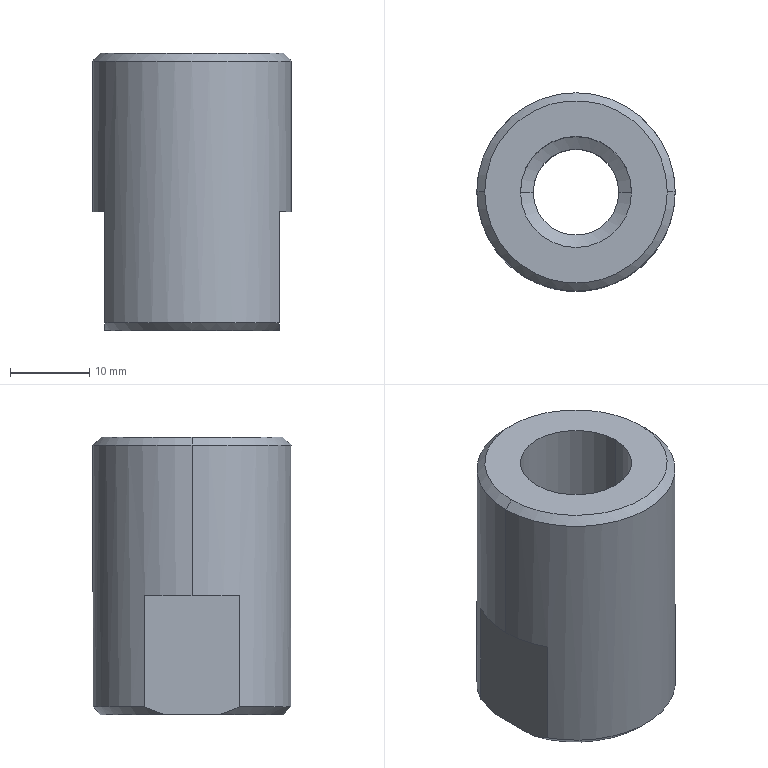Part | STEP file | fBY02F02M-00-13A | 1 solid | 18 faces | box 25 x 25 x 35 mm | volume 12210 mm3 | cylinder 6 | cone 6 | plane 6 | commonest cylinder face diameters 10.8 x2 14 x2 25 x2
STEP:
#1=CARTESIAN_POINT('',(0.,0.,0.));
#2=DIRECTION('',(0.,0.,1.));
#3=DIRECTION('',(1.,0.,0.));
#4=AXIS2_PLACEMENT_3D('',#1,#2,#3);
#5=CARTESIAN_POINT('',(-12.5,0.,34.));
#6=VERTEX_POINT('',#5);
#7=CARTESIAN_POINT('',(12.5,0.,34.));
#8=VERTEX_POINT('',#7);
#9=CARTESIAN_POINT('',(0.,0.,34.));
#10=DIRECTION('',(0.,0.,-1.));
#11=DIRECTION('',(-1.,0.,0.));
#12=AXIS2_PLACEMENT_3D('',#9,#10,#11);
#13=CIRCLE('',#12,12.5);
#14=CARTESIAN_POINT('',(0.,0.,35.));
#15=DIRECTION('',(0.,0.,-1.));
#16=DIRECTION('',(-1.,0.,0.));
#17=AXIS2_PLACEMENT_3D('',#14,#15,#16);
#18=CYLINDRICAL_SURFACE('',#17,12.5);
#19=CARTESIAN_POINT('',(0.,1.));
#20=DIRECTION('',(1.,0.));
#21=VECTOR('',#20,1.);
#22=LINE('',#19,#21);
#23=(GEOMETRIC_REPRESENTATION_CONTEXT(2)PARAMETRIC_REPRESENTATION_CONTEXT()REPRESENTATION_CONTEXT('',''));
#24=DEFINITIONAL_REPRESENTATION('',(#22),#23);
#25=PCURVE('',#18,#24);
#26=CARTESIAN_POINT('',(0.,0.,34.));
#27=DIRECTION('',(0.,0.,-1.));
#28=DIRECTION('',(-1.,0.,0.));
#29=AXIS2_PLACEMENT_3D('',#26,#27,#28);
#30=CONICAL_SURFACE('',#29,12.5,0.7854);
#31=CARTESIAN_POINT('',(0.,0.));
#32=DIRECTION('',(1.,0.));
#33=VECTOR('',#32,1.);
#34=LINE('',#31,#33);
#35=(GEOMETRIC_REPRESENTATION_CONTEXT(2)PARAMETRIC_REPRESENTATION_CONTEXT()REPRESENTATION_CONTEXT('',''));
#36=DEFINITIONAL_REPRESENTATION('',(#34),#35);
#37=PCURVE('',#30,#36);
#38=SURFACE_CURVE('',#13,(#25,#37),.PCURVE_S1.);
#39=EDGE_CURVE('',#6,#8,#38,.T.);
#40=ORIENTED_EDGE('',*,*,#39,.T.);
#41=CARTESIAN_POINT('',(12.5,0.,15.));
#42=VERTEX_POINT('',#41);
#43=CARTESIAN_POINT('',(12.5,0.,35.));
#44=DIRECTION('',(0.,0.,-1.));
#45=VECTOR('',#44,1.);
#46=LINE('',#43,#45);
#47=CARTESIAN_POINT('',(3.142,0.));
#48=DIRECTION('',(0.,1.));
#49=VECTOR('',#48,1.);
#50=LINE('',#47,#49);
#51=(GEOMETRIC_REPRESENTATION_CONTEXT(2)PARAMETRIC_REPRESENTATION_CONTEXT()REPRESENTATION_CONTEXT('',''));
#52=DEFINITIONAL_REPRESENTATION('',(#50),#51);
#53=PCURVE('',#18,#52);
#54=CARTESIAN_POINT('',(0.,0.,35.));
#55=DIRECTION('',(0.,0.,-1.));
#56=DIRECTION('',(-1.,0.,0.));
#57=AXIS2_PLACEMENT_3D('',#54,#55,#56);
#58=CYLINDRICAL_SURFACE('',#57,12.5);
#59=CARTESIAN_POINT('',(3.142,0.));
#60=DIRECTION('',(0.,1.));
#61=VECTOR('',#60,1.);
#62=LINE('',#59,#61);
#63=(GEOMETRIC_REPRESENTATION_CONTEXT(2)PARAMETRIC_REPRESENTATION_CONTEXT()REPRESENTATION_CONTEXT('',''));
#64=DEFINITIONAL_REPRESENTATION('',(#62),#63);
#65=PCURVE('',#58,#64);
#66=SURFACE_CURVE('',#46,(#53,#65),.PCURVE_S1.);
#67=EDGE_CURVE('',#8,#42,#66,.T.);
#68=ORIENTED_EDGE('',*,*,#67,.T.);
#69=CARTESIAN_POINT('',(11.,5.937,15.));
#70=VERTEX_POINT('',#69);
#71=CARTESIAN_POINT('',(0.,0.,15.));
#72=DIRECTION('',(0.,0.,1.));
#73=DIRECTION('',(-1.,0.,0.));
#74=AXIS2_PLACEMENT_3D('',#71,#72,#73);
#75=CIRCLE('',#74,12.5);
#76=CARTESIAN_POINT('',(6.283,20.));
#77=DIRECTION('',(-1.,0.));
#78=VECTOR('',#77,1.);
#79=LINE('',#76,#78);
#80=(GEOMETRIC_REPRESENTATION_CONTEXT(2)PARAMETRIC_REPRESENTATION_CONTEXT()REPRESENTATION_CONTEXT('',''));
#81=DEFINITIONAL_REPRESENTATION('',(#79),#80);
#82=PCURVE('',#18,#81);
#83=CARTESIAN_POINT('',(0.,1.131,15.));
#84=DIRECTION('',(0.,0.,-1.));
#85=DIRECTION('',(-1.,0.,0.));
#86=AXIS2_PLACEMENT_3D('',#83,#84,#85);
#87=PLANE('',#86);
#88=CARTESIAN_POINT('',(12.5,-1.131));
#89=CARTESIAN_POINT('',(12.5,-22.781));
#90=CARTESIAN_POINT('',(-6.25,-11.956));
#91=CARTESIAN_POINT('',(-25.,-1.131));
#92=CARTESIAN_POINT('',(-6.25,9.694));
#93=CARTESIAN_POINT('',(12.5,20.52));
#94=CARTESIAN_POINT('',(12.5,-1.131));
#95=(BOUNDED_CURVE()B_SPLINE_CURVE(2,(#88,#89,#90,#91,#92,#93,#94),.UNSPECIFIED.,.T.,.F.)B_SPLINE_CURVE_WITH_KNOTS((1,2,2,2,2,1),(-2.094,0.,2.094,4.189,6.283,8.378),.UNSPECIFIED.)CURVE()GEOMETRIC_REPRESENTATION_ITEM()RATIONAL_B_SPLINE_CURVE((1.,0.5,1.,0.5,1.,0.5,1.))REPRESENTATION_ITEM(''));
#96=(GEOMETRIC_REPRESENTATION_CONTEXT(2)PARAMETRIC_REPRESENTATION_CONTEXT()REPRESENTATION_CONTEXT('',''));
#97=DEFINITIONAL_REPRESENTATION('',(#95),#96);
#98=PCURVE('',#87,#97);
#99=SURFACE_CURVE('',#75,(#82,#98),.PCURVE_S1.);
#100=EDGE_CURVE('',#42,#70,#99,.T.);
#101=ORIENTED_EDGE('',*,*,#100,.T.);
#102=CARTESIAN_POINT('',(11.,5.937,1.));
#103=VERTEX_POINT('',#102);
#104=CARTESIAN_POINT('',(11.,5.937,35.));
#105=DIRECTION('',(0.,0.,-1.));
#106=VECTOR('',#105,1.);
#107=LINE('',#104,#106);
#108=CARTESIAN_POINT('',(2.647,0.));
#109=DIRECTION('',(0.,1.));
#110=VECTOR('',#109,1.);
#111=LINE('',#108,#110);
#112=(GEOMETRIC_REPRESENTATION_CONTEXT(2)PARAMETRIC_REPRESENTATION_CONTEXT()REPRESENTATION_CONTEXT('',''));
#113=DEFINITIONAL_REPRESENTATION('',(#111),#112);
#114=PCURVE('',#18,#113);
#115=CARTESIAN_POINT('',(11.,15.493,15.));
#116=DIRECTION('',(1.,0.,0.));
#117=DIRECTION('',(0.,1.,0.));
#118=AXIS2_PLACEMENT_3D('',#115,#116,#117);
#119=PLANE('',#118);
#120=CARTESIAN_POINT('',(-9.555,20.));
#121=DIRECTION('',(0.,-1.));
#122=VECTOR('',#121,1.);
#123=LINE('',#120,#122);
#124=(GEOMETRIC_REPRESENTATION_CONTEXT(2)PARAMETRIC_REPRESENTATION_CONTEXT()REPRESENTATION_CONTEXT('',''));
#125=DEFINITIONAL_REPRESENTATION('',(#123),#124);
#126=PCURVE('',#119,#125);
#127=SURFACE_CURVE('',#107,(#114,#126),.PCURVE_S1.);
#128=EDGE_CURVE('',#70,#103,#127,.T.);
#129=ORIENTED_EDGE('',*,*,#128,.T.);
#130=CARTESIAN_POINT('',(-11.,5.937,1.));
#131=VERTEX_POINT('',#130);
#132=CARTESIAN_POINT('',(0.,0.,1.));
#133=DIRECTION('',(0.,0.,1.));
#134=DIRECTION('',(-1.,0.,0.));
#135=AXIS2_PLACEMENT_3D('',#132,#133,#134);
#136=CIRCLE('',#135,12.5);
#137=CARTESIAN_POINT('',(6.283,34.));
#138=DIRECTION('',(-1.,0.));
#139=VECTOR('',#138,1.);
#140=LINE('',#137,#139);
#141=(GEOMETRIC_REPRESENTATION_CONTEXT(2)PARAMETRIC_REPRESENTATION_CONTEXT()REPRESENTATION_CONTEXT('',''));
#142=DEFINITIONAL_REPRESENTATION('',(#140),#141);
#143=PCURVE('',#18,#142);
#144=CARTESIAN_POINT('',(0.,0.,1.));
#145=DIRECTION('',(0.,0.,1.));
#146=DIRECTION('',(1.,0.,0.));
#147=AXIS2_PLACEMENT_3D('',#144,#145,#146);
#148=CONICAL_SURFACE('',#147,12.5,0.7854);
#149=CARTESIAN_POINT('',(-3.142,0.));
#150=DIRECTION('',(1.,0.));
#151=VECTOR('',#150,1.);
#152=LINE('',#149,#151);
#153=(GEOMETRIC_REPRESENTATION_CONTEXT(2)PARAMETRIC_REPRESENTATION_CONTEXT()REPRESENTATION_CONTEXT('',''));
#154=DEFINITIONAL_REPRESENTATION('',(#152),#153);
#155=PCURVE('',#148,#154);
#156=SURFACE_CURVE('',#136,(#143,#155),.PCURVE_S1.);
#157=EDGE_CURVE('',#103,#131,#156,.T.);
#158=ORIENTED_EDGE('',*,*,#157,.T.);
#159=CARTESIAN_POINT('',(-11.,5.937,15.));
#160=VERTEX_POINT('',#159);
#161=CARTESIAN_POINT('',(-11.,5.937,35.));
#162=DIRECTION('',(0.,0.,1.));
#163=VECTOR('',#162,1.);
#164=LINE('',#161,#163);
#165=CARTESIAN_POINT('',(0.4949,0.));
#166=DIRECTION('',(0.,-1.));
#167=VECTOR('',#166,1.);
#168=LINE('',#165,#167);
#169=(GEOMETRIC_REPRESENTATION_CONTEXT(2)PARAMETRIC_REPRESENTATION_CONTEXT()REPRESENTATION_CONTEXT('',''));
#170=DEFINITIONAL_REPRESENTATION('',(#168),#169);
#171=PCURVE('',#18,#170);
#172=CARTESIAN_POINT('',(-11.,15.493,15.));
#173=DIRECTION('',(-1.,0.,0.));
#174=DIRECTION('',(0.,-1.,0.));
#175=AXIS2_PLACEMENT_3D('',#172,#173,#174);
#176=PLANE('',#175);
#177=CARTESIAN_POINT('',(9.555,20.));
#178=DIRECTION('',(0.,1.));
#179=VECTOR('',#178,1.);
#180=LINE('',#177,#179);
#181=(GEOMETRIC_REPRESENTATION_CONTEXT(2)PARAMETRIC_REPRESENTATION_CONTEXT()REPRESENTATION_CONTEXT('',''));
#182=DEFINITIONAL_REPRESENTATION('',(#180),#181);
#183=PCURVE('',#176,#182);
#184=SURFACE_CURVE('',#164,(#171,#183),.PCURVE_S1.);
#185=EDGE_CURVE('',#131,#160,#184,.T.);
#186=ORIENTED_EDGE('',*,*,#185,.T.);
#187=CARTESIAN_POINT('',(-12.5,0.,15.));
#188=VERTEX_POINT('',#187);
#189=CARTESIAN_POINT('',(0.,0.,15.));
#190=DIRECTION('',(0.,0.,1.));
#191=DIRECTION('',(-1.,0.,0.));
#192=AXIS2_PLACEMENT_3D('',#189,#190,#191);
#193=CIRCLE('',#192,12.5);
#194=CARTESIAN_POINT('',(6.283,20.));
#195=DIRECTION('',(-1.,0.));
#196=VECTOR('',#195,1.);
#197=LINE('',#194,#196);
#198=(GEOMETRIC_REPRESENTATION_CONTEXT(2)PARAMETRIC_REPRESENTATION_CONTEXT()REPRESENTATION_CONTEXT('',''));
#199=DEFINITIONAL_REPRESENTATION('',(#197),#198);
#200=PCURVE('',#18,#199);
#201=CARTESIAN_POINT('',(0.,1.131,15.));
#202=DIRECTION('',(0.,0.,-1.));
#203=DIRECTION('',(-1.,0.,0.));
#204=AXIS2_PLACEMENT_3D('',#201,#202,#203);
#205=PLANE('',#204);
#206=CARTESIAN_POINT('',(12.5,-1.131));
#207=CARTESIAN_POINT('',(12.5,-22.781));
#208=CARTESIAN_POINT('',(-6.25,-11.956));
#209=CARTESIAN_POINT('',(-25.,-1.131));
#210=CARTESIAN_POINT('',(-6.25,9.694));
#211=CARTESIAN_POINT('',(12.5,20.52));
#212=CARTESIAN_POINT('',(12.5,-1.131));
#213=(BOUNDED_CURVE()B_SPLINE_CURVE(2,(#206,#207,#208,#209,#210,#211,#212),.UNSPECIFIED.,.T.,.F.)B_SPLINE_CURVE_WITH_KNOTS((1,2,2,2,2,1),(-2.094,0.,2.094,4.189,6.283,8.378),.UNSPECIFIED.)CURVE()GEOMETRIC_REPRESENTATION_ITEM()RATIONAL_B_SPLINE_CURVE((1.,0.5,1.,0.5,1.,0.5,1.))REPRESENTATION_ITEM(''));
#214=(GEOMETRIC_REPRESENTATION_CONTEXT(2)PARAMETRIC_REPRESENTATION_CONTEXT()REPRESENTATION_CONTEXT('',''));
#215=DEFINITIONAL_REPRESENTATION('',(#213),#214);
#216=PCURVE('',#205,#215);
#217=SURFACE_CURVE('',#193,(#200,#216),.PCURVE_S1.);
#218=EDGE_CURVE('',#160,#188,#217,.T.);
#219=ORIENTED_EDGE('',*,*,#218,.T.);
#220=CARTESIAN_POINT('',(-12.5,0.,35.));
#221=DIRECTION('',(0.,0.,-1.));
#222=VECTOR('',#221,1.);
#223=LINE('',#220,#222);
#224=CARTESIAN_POINT('',(0.,0.));
#225=DIRECTION('',(0.,1.));
#226=VECTOR('',#225,1.);
#227=LINE('',#224,#226);
#228=(GEOMETRIC_REPRESENTATION_CONTEXT(2)PARAMETRIC_REPRESENTATION_CONTEXT()REPRESENTATION_CONTEXT('',''));
#229=DEFINITIONAL_REPRESENTATION('',(#227),#228);
#230=PCURVE('',#18,#229);
#231=CARTESIAN_POINT('',(6.283,0.));
#232=DIRECTION('',(0.,1.));
#233=VECTOR('',#232,1.);
#234=LINE('',#231,#233);
#235=(GEOMETRIC_REPRESENTATION_CONTEXT(2)PARAMETRIC_REPRESENTATION_CONTEXT()REPRESENTATION_CONTEXT('',''));
#236=DEFINITIONAL_REPRESENTATION('',(#234),#235);
#237=PCURVE('',#58,#236);
#238=SURFACE_CURVE('',#223,(#230,#237),.PCURVE_S1.);
#239=EDGE_CURVE('',#6,#188,#238,.T.);
#240=ORIENTED_EDGE('',*,*,#239,.F.);
#241=EDGE_LOOP('',(#40,#68,#101,#129,#158,#186,#219,#240));
#242=FACE_BOUND('',#241,.T.);
#243=ADVANCED_FACE('',(#242),#18,.T.);
#244=CARTESIAN_POINT('',(-11.5,0.,35.));
#245=VERTEX_POINT('',#244);
#246=CARTESIAN_POINT('',(11.5,0.,35.));
#247=VERTEX_POINT('',#246);
#248=CARTESIAN_POINT('',(0.,0.,35.));
#249=DIRECTION('',(0.,0.,-1.));
#250=DIRECTION('',(-1.,0.,0.));
#251=AXIS2_PLACEMENT_3D('',#248,#249,#250);
#252=CIRCLE('',#251,11.5);
#253=CARTESIAN_POINT('',(0.,-1.));
#254=DIRECTION('',(1.,0.));
#255=VECTOR('',#254,1.);
#256=LINE('',#253,#255);
#257=(GEOMETRIC_REPRESENTATION_CONTEXT(2)PARAMETRIC_REPRESENTATION_CONTEXT()REPRESENTATION_CONTEXT('',''));
#258=DEFINITIONAL_REPRESENTATION('',(#256),#257);
#259=PCURVE('',#30,#258);
#260=CARTESIAN_POINT('',(0.,0.,35.));
#261=DIRECTION('',(0.,0.,1.));
#262=DIRECTION('',(1.,0.,0.));
#263=AXIS2_PLACEMENT_3D('',#260,#261,#262);
#264=PLANE('',#263);
#265=CARTESIAN_POINT('',(-11.5,0.));
#266=CARTESIAN_POINT('',(-11.5,19.919));
#267=CARTESIAN_POINT('',(5.75,9.959));
#268=CARTESIAN_POINT('',(23.,0.));
#269=CARTESIAN_POINT('',(5.75,-9.959));
#270=CARTESIAN_POINT('',(-11.5,-19.919));
#271=CARTESIAN_POINT('',(-11.5,0.));
#272=(BOUNDED_CURVE()B_SPLINE_CURVE(2,(#265,#266,#267,#268,#269,#270,#271),.UNSPECIFIED.,.T.,.F.)B_SPLINE_CURVE_WITH_KNOTS((1,2,2,2,2,1),(-2.094,0.,2.094,4.189,6.283,8.378),.UNSPECIFIED.)CURVE()GEOMETRIC_REPRESENTATION_ITEM()RATIONAL_B_SPLINE_CURVE((1.,0.5,1.,0.5,1.,0.5,1.))REPRESENTATION_ITEM(''));
#273=(GEOMETRIC_REPRESENTATION_CONTEXT(2)PARAMETRIC_REPRESENTATION_CONTEXT()REPRESENTATION_CONTEXT('',''));
#274=DEFINITIONAL_REPRESENTATION('',(#272),#273);
#275=PCURVE('',#264,#274);
#276=SURFACE_CURVE('',#252,(#259,#275),.PCURVE_S1.);
#277=EDGE_CURVE('',#245,#247,#276,.T.);
#278=ORIENTED_EDGE('',*,*,#277,.T.);
#279=CARTESIAN_POINT('',(12.5,0.,34.));
#280=DIRECTION('',(0.7071,0.,-0.7071));
#281=VECTOR('',#280,1.);
#282=LINE('',#279,#281);
#283=CARTESIAN_POINT('',(3.142,0.));
#284=DIRECTION('',(0.,1.));
#285=VECTOR('',#284,1.);
#286=LINE('',#283,#285);
#287=(GEOMETRIC_REPRESENTATION_CONTEXT(2)PARAMETRIC_REPRESENTATION_CONTEXT()REPRESENTATION_CONTEXT('',''));
#288=DEFINITIONAL_REPRESENTATION('',(#286),#287);
#289=PCURVE('',#30,#288);
#290=CARTESIAN_POINT('',(0.,0.,34.));
#291=DIRECTION('',(0.,0.,-1.));
#292=DIRECTION('',(-1.,0.,0.));
#293=AXIS2_PLACEMENT_3D('',#290,#291,#292);
#294=CONICAL_SURFACE('',#293,12.5,0.7854);
#295=CARTESIAN_POINT('',(3.142,0.));
#296=DIRECTION('',(0.,1.));
#297=VECTOR('',#296,1.);
#298=LINE('',#295,#297);
#299=(GEOMETRIC_REPRESENTATION_CONTEXT(2)PARAMETRIC_REPRESENTATION_CONTEXT()REPRESENTATION_CONTEXT('',''));
#300=DEFINITIONAL_REPRESENTATION('',(#298),#299);
#301=PCURVE('',#294,#300);
#302=SURFACE_CURVE('',#282,(#289,#301),.PCURVE_S1.);
#303=EDGE_CURVE('',#247,#8,#302,.T.);
#304=ORIENTED_EDGE('',*,*,#303,.T.);
#305=ORIENTED_EDGE('',*,*,#39,.F.);
#306=CARTESIAN_POINT('',(-12.5,0.,34.));
#307=DIRECTION('',(-0.7071,0.,-0.7071));
#308=VECTOR('',#307,1.);
#309=LINE('',#306,#308);
#310=CARTESIAN_POINT('',(0.,0.));
#311=DIRECTION('',(0.,1.));
#312=VECTOR('',#311,1.);
#313=LINE('',#310,#312);
#314=(GEOMETRIC_REPRESENTATION_CONTEXT(2)PARAMETRIC_REPRESENTATION_CONTEXT()REPRESENTATION_CONTEXT('',''));
#315=DEFINITIONAL_REPRESENTATION('',(#313),#314);
#316=PCURVE('',#30,#315);
#317=CARTESIAN_POINT('',(6.283,0.));
#318=DIRECTION('',(0.,1.));
#319=VECTOR('',#318,1.);
#320=LINE('',#317,#319);
#321=(GEOMETRIC_REPRESENTATION_CONTEXT(2)PARAMETRIC_REPRESENTATION_CONTEXT()REPRESENTATION_CONTEXT('',''));
#322=DEFINITIONAL_REPRESENTATION('',(#320),#321);
#323=PCURVE('',#294,#322);
#324=SURFACE_CURVE('',#309,(#316,#323),.PCURVE_S1.);
#325=EDGE_CURVE('',#245,#6,#324,.T.);
#326=ORIENTED_EDGE('',*,*,#325,.F.);
#327=EDGE_LOOP('',(#278,#304,#305,#326));
#328=FACE_BOUND('',#327,.T.);
#329=ADVANCED_FACE('',(#328),#30,.T.);
#330=CARTESIAN_POINT('',(-5.4,0.,13.039));
#331=VERTEX_POINT('',#330);
#332=CARTESIAN_POINT('',(-5.4,0.,0.));
#333=VERTEX_POINT('',#332);
#334=CARTESIAN_POINT('',(-5.4,0.,0.));
#335=DIRECTION('',(0.,0.,-1.));
#336=VECTOR('',#335,1.);
#337=LINE('',#334,#336);
#338=CARTESIAN_POINT('',(0.,0.,0.));
#339=DIRECTION('',(0.,0.,-1.));
#340=DIRECTION('',(-1.,0.,0.));
#341=AXIS2_PLACEMENT_3D('',#338,#339,#340);
#342=CYLINDRICAL_SURFACE('',#341,5.4);
#343=CARTESIAN_POINT('',(6.283,0.));
#344=DIRECTION('',(0.,1.));
#345=VECTOR('',#344,1.);
#346=LINE('',#343,#345);
#347=(GEOMETRIC_REPRESENTATION_CONTEXT(2)PARAMETRIC_REPRESENTATION_CONTEXT()REPRESENTATION_CONTEXT('',''));
#348=DEFINITIONAL_REPRESENTATION('',(#346),#347);
#349=PCURVE('',#342,#348);
#350=CARTESIAN_POINT('',(0.,0.,0.));
#351=DIRECTION('',(0.,0.,-1.));
#352=DIRECTION('',(-1.,0.,0.));
#353=AXIS2_PLACEMENT_3D('',#350,#351,#352);
#354=CYLINDRICAL_SURFACE('',#353,5.4);
#355=CARTESIAN_POINT('',(0.,0.));
#356=DIRECTION('',(0.,1.));
#357=VECTOR('',#356,1.);
#358=LINE('',#355,#357);
#359=(GEOMETRIC_REPRESENTATION_CONTEXT(2)PARAMETRIC_REPRESENTATION_CONTEXT()REPRESENTATION_CONTEXT('',''));
#360=DEFINITIONAL_REPRESENTATION('',(#358),#359);
#361=PCURVE('',#354,#360);
#362=SURFACE_CURVE('',#337,(#349,#361),.PCURVE_S1.);
#363=EDGE_CURVE('',#331,#333,#362,.T.);
#364=ORIENTED_EDGE('',*,*,#363,.T.);
#365=CARTESIAN_POINT('',(5.4,0.,0.));
#366=VERTEX_POINT('',#365);
#367=CARTESIAN_POINT('',(0.,0.,0.));
#368=DIRECTION('',(0.,0.,-1.));
#369=DIRECTION('',(-1.,0.,0.));
#370=AXIS2_PLACEMENT_3D('',#367,#368,#369);
#371=CIRCLE('',#370,5.4);
#372=CARTESIAN_POINT('',(0.,0.));
#373=DIRECTION('',(1.,0.));
#374=VECTOR('',#373,1.);
#375=LINE('',#372,#374);
#376=(GEOMETRIC_REPRESENTATION_CONTEXT(2)PARAMETRIC_REPRESENTATION_CONTEXT()REPRESENTATION_CONTEXT('',''));
#377=DEFINITIONAL_REPRESENTATION('',(#375),#376);
#378=PCURVE('',#342,#377);
#379=CARTESIAN_POINT('',(0.,0.,0.));
#380=DIRECTION('',(0.,0.,1.));
#381=DIRECTION('',(1.,0.,0.));
#382=AXIS2_PLACEMENT_3D('',#379,#380,#381);
#383=PLANE('',#382);
#384=CARTESIAN_POINT('',(-5.4,0.));
#385=CARTESIAN_POINT('',(-5.4,9.353));
#386=CARTESIAN_POINT('',(2.7,4.677));
#387=CARTESIAN_POINT('',(10.8,0.));
#388=CARTESIAN_POINT('',(2.7,-4.677));
#389=CARTESIAN_POINT('',(-5.4,-9.353));
#390=CARTESIAN_POINT('',(-5.4,0.));
#391=(BOUNDED_CURVE()B_SPLINE_CURVE(2,(#384,#385,#386,#387,#388,#389,#390),.UNSPECIFIED.,.T.,.F.)B_SPLINE_CURVE_WITH_KNOTS((1,2,2,2,2,1),(-2.094,0.,2.094,4.189,6.283,8.378),.UNSPECIFIED.)CURVE()GEOMETRIC_REPRESENTATION_ITEM()RATIONAL_B_SPLINE_CURVE((1.,0.5,1.,0.5,1.,0.5,1.))REPRESENTATION_ITEM(''));
#392=(GEOMETRIC_REPRESENTATION_CONTEXT(2)PARAMETRIC_REPRESENTATION_CONTEXT()REPRESENTATION_CONTEXT('',''));
#393=DEFINITIONAL_REPRESENTATION('',(#391),#392);
#394=PCURVE('',#383,#393);
#395=SURFACE_CURVE('',#371,(#378,#394),.PCURVE_S1.);
#396=EDGE_CURVE('',#366,#333,#395,.T.);
#397=ORIENTED_EDGE('',*,*,#396,.F.);
#398=CARTESIAN_POINT('',(5.4,0.,13.039));
#399=VERTEX_POINT('',#398);
#400=CARTESIAN_POINT('',(5.4,0.,0.));
#401=DIRECTION('',(0.,0.,-1.));
#402=VECTOR('',#401,1.);
#403=LINE('',#400,#402);
#404=CARTESIAN_POINT('',(3.142,0.));
#405=DIRECTION('',(0.,1.));
#406=VECTOR('',#405,1.);
#407=LINE('',#404,#406);
#408=(GEOMETRIC_REPRESENTATION_CONTEXT(2)PARAMETRIC_REPRESENTATION_CONTEXT()REPRESENTATION_CONTEXT('',''));
#409=DEFINITIONAL_REPRESENTATION('',(#407),#408);
#410=PCURVE('',#342,#409);
#411=CARTESIAN_POINT('',(3.142,0.));
#412=DIRECTION('',(0.,1.));
#413=VECTOR('',#412,1.);
#414=LINE('',#411,#413);
#415=(GEOMETRIC_REPRESENTATION_CONTEXT(2)PARAMETRIC_REPRESENTATION_CONTEXT()REPRESENTATION_CONTEXT('',''));
#416=DEFINITIONAL_REPRESENTATION('',(#414),#415);
#417=PCURVE('',#354,#416);
#418=SURFACE_CURVE('',#403,(#410,#417),.PCURVE_S1.);
#419=EDGE_CURVE('',#399,#366,#418,.T.);
#420=ORIENTED_EDGE('',*,*,#419,.F.);
#421=CARTESIAN_POINT('',(0.,0.,13.039));
#422=DIRECTION('',(0.,0.,-1.));
#423=DIRECTION('',(-1.,0.,0.));
#424=AXIS2_PLACEMENT_3D('',#421,#422,#423);
#425=CIRCLE('',#424,5.4);
#426=CARTESIAN_POINT('',(0.,-13.039));
#427=DIRECTION('',(1.,0.));
#428=VECTOR('',#427,1.);
#429=LINE('',#426,#428);
#430=(GEOMETRIC_REPRESENTATION_CONTEXT(2)PARAMETRIC_REPRESENTATION_CONTEXT()REPRESENTATION_CONTEXT('',''));
#431=DEFINITIONAL_REPRESENTATION('',(#429),#430);
#432=PCURVE('',#342,#431);
#433=CARTESIAN_POINT('',(0.,0.,14.));
#434=DIRECTION('',(0.,0.,1.));
#435=DIRECTION('',(1.,0.,0.));
#436=AXIS2_PLACEMENT_3D('',#433,#434,#435);
#437=CONICAL_SURFACE('',#436,7.,1.03);
#438=CARTESIAN_POINT('',(9.425,-0.9614));
#439=DIRECTION('',(-1.,0.));
#440=VECTOR('',#439,1.);
#441=LINE('',#438,#440);
#442=(GEOMETRIC_REPRESENTATION_CONTEXT(2)PARAMETRIC_REPRESENTATION_CONTEXT()REPRESENTATION_CONTEXT('',''));
#443=DEFINITIONAL_REPRESENTATION('',(#441),#442);
#444=PCURVE('',#437,#443);
#445=SURFACE_CURVE('',#425,(#432,#444),.PCURVE_S1.);
#446=EDGE_CURVE('',#399,#331,#445,.T.);
#447=ORIENTED_EDGE('',*,*,#446,.T.);
#448=EDGE_LOOP('',(#364,#397,#420,#447));
#449=FACE_BOUND('',#448,.F.);
#450=ADVANCED_FACE('',(#449),#342,.F.);
#451=CARTESIAN_POINT('',(7.,0.,14.));
#452=VERTEX_POINT('',#451);
#453=CARTESIAN_POINT('',(7.,0.,35.));
#454=VERTEX_POINT('',#453);
#455=CARTESIAN_POINT('',(7.,0.,35.));
#456=DIRECTION('',(0.,0.,1.));
#457=VECTOR('',#456,1.);
#458=LINE('',#455,#457);
#459=CARTESIAN_POINT('',(0.,0.,35.));
#460=DIRECTION('',(0.,0.,1.));
#461=DIRECTION('',(1.,0.,0.));
#462=AXIS2_PLACEMENT_3D('',#459,#460,#461);
#463=CYLINDRICAL_SURFACE('',#462,7.);
#464=CARTESIAN_POINT('',(6.283,0.));
#465=DIRECTION('',(0.,1.));
#466=VECTOR('',#465,1.);
#467=LINE('',#464,#466);
#468=(GEOMETRIC_REPRESENTATION_CONTEXT(2)PARAMETRIC_REPRESENTATION_CONTEXT()REPRESENTATION_CONTEXT('',''));
#469=DEFINITIONAL_REPRESENTATION('',(#467),#468);
#470=PCURVE('',#463,#469);
#471=CARTESIAN_POINT('',(0.,0.,35.));
#472=DIRECTION('',(0.,0.,1.));
#473=DIRECTION('',(1.,0.,0.));
#474=AXIS2_PLACEMENT_3D('',#471,#472,#473);
#475=CYLINDRICAL_SURFACE('',#474,7.);
#476=CARTESIAN_POINT('',(0.,0.));
#477=DIRECTION('',(0.,1.));
#478=VECTOR('',#477,1.);
#479=LINE('',#476,#478);
#480=(GEOMETRIC_REPRESENTATION_CONTEXT(2)PARAMETRIC_REPRESENTATION_CONTEXT()REPRESENTATION_CONTEXT('',''));
#481=DEFINITIONAL_REPRESENTATION('',(#479),#480);
#482=PCURVE('',#475,#481);
#483=SURFACE_CURVE('',#458,(#470,#482),.PCURVE_S1.);
#484=EDGE_CURVE('',#452,#454,#483,.T.);
#485=ORIENTED_EDGE('',*,*,#484,.T.);
#486=CARTESIAN_POINT('',(-7.,0.,35.));
#487=VERTEX_POINT('',#486);
#488=CARTESIAN_POINT('',(0.,0.,35.));
#489=DIRECTION('',(0.,0.,-1.));
#490=DIRECTION('',(1.,0.,0.));
#491=AXIS2_PLACEMENT_3D('',#488,#489,#490);
#492=CIRCLE('',#491,7.);
#493=CARTESIAN_POINT('',(6.283,0.));
#494=DIRECTION('',(-1.,0.));
#495=VECTOR('',#494,1.);
#496=LINE('',#493,#495);
#497=(GEOMETRIC_REPRESENTATION_CONTEXT(2)PARAMETRIC_REPRESENTATION_CONTEXT()REPRESENTATION_CONTEXT('',''));
#498=DEFINITIONAL_REPRESENTATION('',(#496),#497);
#499=PCURVE('',#463,#498);
#500=CARTESIAN_POINT('',(7.,0.));
#501=CARTESIAN_POINT('',(7.,-12.124));
#502=CARTESIAN_POINT('',(-3.5,-6.062));
#503=CARTESIAN_POINT('',(-14.,0.));
#504=CARTESIAN_POINT('',(-3.5,6.062));
#505=CARTESIAN_POINT('',(7.,12.124));
#506=CARTESIAN_POINT('',(7.,0.));
#507=(BOUNDED_CURVE()B_SPLINE_CURVE(2,(#500,#501,#502,#503,#504,#505,#506),.UNSPECIFIED.,.T.,.F.)B_SPLINE_CURVE_WITH_KNOTS((1,2,2,2,2,1),(-2.094,0.,2.094,4.189,6.283,8.378),.UNSPECIFIED.)CURVE()GEOMETRIC_REPRESENTATION_ITEM()RATIONAL_B_SPLINE_CURVE((1.,0.5,1.,0.5,1.,0.5,1.))REPRESENTATION_ITEM(''));
#508=(GEOMETRIC_REPRESENTATION_CONTEXT(2)PARAMETRIC_REPRESENTATION_CONTEXT()REPRESENTATION_CONTEXT('',''));
#509=DEFINITIONAL_REPRESENTATION('',(#507),#508);
#510=PCURVE('',#264,#509);
#511=SURFACE_CURVE('',#492,(#499,#510),.PCURVE_S1.);
#512=EDGE_CURVE('',#454,#487,#511,.T.);
#513=ORIENTED_EDGE('',*,*,#512,.T.);
#514=CARTESIAN_POINT('',(-7.,0.,14.));
#515=VERTEX_POINT('',#514);
#516=CARTESIAN_POINT('',(-7.,0.,35.));
#517=DIRECTION('',(0.,0.,1.));
#518=VECTOR('',#517,1.);
#519=LINE('',#516,#518);
#520=CARTESIAN_POINT('',(3.142,0.));
#521=DIRECTION('',(0.,1.));
#522=VECTOR('',#521,1.);
#523=LINE('',#520,#522);
#524=(GEOMETRIC_REPRESENTATION_CONTEXT(2)PARAMETRIC_REPRESENTATION_CONTEXT()REPRESENTATION_CONTEXT('',''));
#525=DEFINITIONAL_REPRESENTATION('',(#523),#524);
#526=PCURVE('',#463,#525);
#527=CARTESIAN_POINT('',(3.142,0.));
#528=DIRECTION('',(0.,1.));
#529=VECTOR('',#528,1.);
#530=LINE('',#527,#529);
#531=(GEOMETRIC_REPRESENTATION_CONTEXT(2)PARAMETRIC_REPRESENTATION_CONTEXT()REPRESENTATION_CONTEXT('',''));
#532=DEFINITIONAL_REPRESENTATION('',(#530),#531);
#533=PCURVE('',#475,#532);
#534=SURFACE_CURVE('',#519,(#526,#533),.PCURVE_S1.);
#535=EDGE_CURVE('',#515,#487,#534,.T.);
#536=ORIENTED_EDGE('',*,*,#535,.F.);
#537=CARTESIAN_POINT('',(0.,0.,14.));
#538=DIRECTION('',(0.,0.,1.));
#539=DIRECTION('',(1.,0.,0.));
#540=AXIS2_PLACEMENT_3D('',#537,#538,#539);
#541=CIRCLE('',#540,7.);
#542=CARTESIAN_POINT('',(0.,-21.));
#543=DIRECTION('',(1.,0.));
#544=VECTOR('',#543,1.);
#545=LINE('',#542,#544);
#546=(GEOMETRIC_REPRESENTATION_CONTEXT(2)PARAMETRIC_REPRESENTATION_CONTEXT()REPRESENTATION_CONTEXT('',''));
#547=DEFINITIONAL_REPRESENTATION('',(#545),#546);
#548=PCURVE('',#463,#547);
#549=CARTESIAN_POINT('',(0.,0.));
#550=DIRECTION('',(1.,0.));
#551=VECTOR('',#550,1.);
#552=LINE('',#549,#551);
#553=(GEOMETRIC_REPRESENTATION_CONTEXT(2)PARAMETRIC_REPRESENTATION_CONTEXT()REPRESENTATION_CONTEXT('',''));
#554=DEFINITIONAL_REPRESENTATION('',(#552),#553);
#555=PCURVE('',#437,#554);
#556=SURFACE_CURVE('',#541,(#548,#555),.PCURVE_S1.);
#557=EDGE_CURVE('',#515,#452,#556,.T.);
#558=ORIENTED_EDGE('',*,*,#557,.T.);
#559=EDGE_LOOP('',(#485,#513,#536,#558));
#560=FACE_BOUND('',#559,.F.);
#561=ADVANCED_FACE('',(#560),#463,.F.);
#562=CARTESIAN_POINT('',(7.,0.,14.));
#563=DIRECTION('',(0.8572,0.,0.515));
#564=VECTOR('',#563,1.);
#565=LINE('',#562,#564);
#566=CARTESIAN_POINT('',(6.283,0.));
#567=DIRECTION('',(0.,1.));
#568=VECTOR('',#567,1.);
#569=LINE('',#566,#568);
#570=(GEOMETRIC_REPRESENTATION_CONTEXT(2)PARAMETRIC_REPRESENTATION_CONTEXT()REPRESENTATION_CONTEXT('',''));
#571=DEFINITIONAL_REPRESENTATION('',(#569),#570);
#572=PCURVE('',#437,#571);
#573=CARTESIAN_POINT('',(0.,0.,14.));
#574=DIRECTION('',(0.,0.,1.));
#575=DIRECTION('',(1.,0.,0.));
#576=AXIS2_PLACEMENT_3D('',#573,#574,#575);
#577=CONICAL_SURFACE('',#576,7.,1.03);
#578=CARTESIAN_POINT('',(0.,0.));
#579=DIRECTION('',(0.,1.));
#580=VECTOR('',#579,1.);
#581=LINE('',#578,#580);
#582=(GEOMETRIC_REPRESENTATION_CONTEXT(2)PARAMETRIC_REPRESENTATION_CONTEXT()REPRESENTATION_CONTEXT('',''));
#583=DEFINITIONAL_REPRESENTATION('',(#581),#582);
#584=PCURVE('',#577,#583);
#585=SURFACE_CURVE('',#565,(#572,#584),.PCURVE_S1.);
#586=EDGE_CURVE('',#399,#452,#585,.T.);
#587=ORIENTED_EDGE('',*,*,#586,.T.);
#588=ORIENTED_EDGE('',*,*,#557,.F.);
#589=CARTESIAN_POINT('',(-7.,0.,14.));
#590=DIRECTION('',(-0.8572,0.,0.515));
#591=VECTOR('',#590,1.);
#592=LINE('',#589,#591);
#593=CARTESIAN_POINT('',(3.142,0.));
#594=DIRECTION('',(0.,1.));
#595=VECTOR('',#594,1.);
#596=LINE('',#593,#595);
#597=(GEOMETRIC_REPRESENTATION_CONTEXT(2)PARAMETRIC_REPRESENTATION_CONTEXT()REPRESENTATION_CONTEXT('',''));
#598=DEFINITIONAL_REPRESENTATION('',(#596),#597);
#599=PCURVE('',#437,#598);
#600=CARTESIAN_POINT('',(3.142,0.));
#601=DIRECTION('',(0.,1.));
#602=VECTOR('',#601,1.);
#603=LINE('',#600,#602);
#604=(GEOMETRIC_REPRESENTATION_CONTEXT(2)PARAMETRIC_REPRESENTATION_CONTEXT()REPRESENTATION_CONTEXT('',''));
#605=DEFINITIONAL_REPRESENTATION('',(#603),#604);
#606=PCURVE('',#577,#605);
#607=SURFACE_CURVE('',#592,(#599,#606),.PCURVE_S1.);
#608=EDGE_CURVE('',#331,#515,#607,.T.);
#609=ORIENTED_EDGE('',*,*,#608,.F.);
#610=ORIENTED_EDGE('',*,*,#446,.F.);
#611=EDGE_LOOP('',(#587,#588,#609,#610));
#612=FACE_BOUND('',#611,.F.);
#613=ADVANCED_FACE('',(#612),#437,.F.);
#614=ORIENTED_EDGE('',*,*,#67,.F.);
#615=CARTESIAN_POINT('',(0.,0.,34.));
#616=DIRECTION('',(0.,0.,-1.));
#617=DIRECTION('',(-1.,0.,0.));
#618=AXIS2_PLACEMENT_3D('',#615,#616,#617);
#619=CIRCLE('',#618,12.5);
#620=CARTESIAN_POINT('',(0.,1.));
#621=DIRECTION('',(1.,0.));
#622=VECTOR('',#621,1.);
#623=LINE('',#620,#622);
#624=(GEOMETRIC_REPRESENTATION_CONTEXT(2)PARAMETRIC_REPRESENTATION_CONTEXT()REPRESENTATION_CONTEXT('',''));
#625=DEFINITIONAL_REPRESENTATION('',(#623),#624);
#626=PCURVE('',#58,#625);
#627=CARTESIAN_POINT('',(0.,0.));
#628=DIRECTION('',(1.,0.));
#629=VECTOR('',#628,1.);
#630=LINE('',#627,#629);
#631=(GEOMETRIC_REPRESENTATION_CONTEXT(2)PARAMETRIC_REPRESENTATION_CONTEXT()REPRESENTATION_CONTEXT('',''));
#632=DEFINITIONAL_REPRESENTATION('',(#630),#631);
#633=PCURVE('',#294,#632);
#634=SURFACE_CURVE('',#619,(#626,#633),.PCURVE_S1.);
#635=EDGE_CURVE('',#8,#6,#634,.T.);
#636=ORIENTED_EDGE('',*,*,#635,.T.);
#637=ORIENTED_EDGE('',*,*,#239,.T.);
#638=CARTESIAN_POINT('',(-11.,-5.937,15.));
#639=VERTEX_POINT('',#638);
#640=CARTESIAN_POINT('',(0.,0.,15.));
#641=DIRECTION('',(0.,0.,1.));
#642=DIRECTION('',(-1.,0.,0.));
#643=AXIS2_PLACEMENT_3D('',#640,#641,#642);
#644=CIRCLE('',#643,12.5);
#645=CARTESIAN_POINT('',(6.283,20.));
#646=DIRECTION('',(-1.,0.));
#647=VECTOR('',#646,1.);
#648=LINE('',#645,#647);
#649=(GEOMETRIC_REPRESENTATION_CONTEXT(2)PARAMETRIC_REPRESENTATION_CONTEXT()REPRESENTATION_CONTEXT('',''));
#650=DEFINITIONAL_REPRESENTATION('',(#648),#649);
#651=PCURVE('',#58,#650);
#652=CARTESIAN_POINT('',(12.5,-1.131));
#653=CARTESIAN_POINT('',(12.5,-22.781));
#654=CARTESIAN_POINT('',(-6.25,-11.956));
#655=CARTESIAN_POINT('',(-25.,-1.131));
#656=CARTESIAN_POINT('',(-6.25,9.694));
#657=CARTESIAN_POINT('',(12.5,20.52));
#658=CARTESIAN_POINT('',(12.5,-1.131));
#659=(BOUNDED_CURVE()B_SPLINE_CURVE(2,(#652,#653,#654,#655,#656,#657,#658),.UNSPECIFIED.,.T.,.F.)B_SPLINE_CURVE_WITH_KNOTS((1,2,2,2,2,1),(-2.094,0.,2.094,4.189,6.283,8.378),.UNSPECIFIED.)CURVE()GEOMETRIC_REPRESENTATION_ITEM()RATIONAL_B_SPLINE_CURVE((1.,0.5,1.,0.5,1.,0.5,1.))REPRESENTATION_ITEM(''));
#660=(GEOMETRIC_REPRESENTATION_CONTEXT(2)PARAMETRIC_REPRESENTATION_CONTEXT()REPRESENTATION_CONTEXT('',''));
#661=DEFINITIONAL_REPRESENTATION('',(#659),#660);
#662=PCURVE('',#205,#661);
#663=SURFACE_CURVE('',#644,(#651,#662),.PCURVE_S1.);
#664=EDGE_CURVE('',#188,#639,#663,.T.);
#665=ORIENTED_EDGE('',*,*,#664,.T.);
#666=CARTESIAN_POINT('',(-11.,-5.937,1.));
#667=VERTEX_POINT('',#666);
#668=CARTESIAN_POINT('',(-11.,-5.937,35.));
#669=DIRECTION('',(0.,0.,-1.));
#670=VECTOR('',#669,1.);
#671=LINE('',#668,#670);
#672=CARTESIAN_POINT('',(5.788,0.));
#673=DIRECTION('',(0.,1.));
#674=VECTOR('',#673,1.);
#675=LINE('',#672,#674);
#676=(GEOMETRIC_REPRESENTATION_CONTEXT(2)PARAMETRIC_REPRESENTATION_CONTEXT()REPRESENTATION_CONTEXT('',''));
#677=DEFINITIONAL_REPRESENTATION('',(#675),#676);
#678=PCURVE('',#58,#677);
#679=CARTESIAN_POINT('',(21.43,20.));
#680=DIRECTION('',(0.,-1.));
#681=VECTOR('',#680,1.);
#682=LINE('',#679,#681);
#683=(GEOMETRIC_REPRESENTATION_CONTEXT(2)PARAMETRIC_REPRESENTATION_CONTEXT()REPRESENTATION_CONTEXT('',''));
#684=DEFINITIONAL_REPRESENTATION('',(#682),#683);
#685=PCURVE('',#176,#684);
#686=SURFACE_CURVE('',#671,(#678,#685),.PCURVE_S1.);
#687=EDGE_CURVE('',#639,#667,#686,.T.);
#688=ORIENTED_EDGE('',*,*,#687,.T.);
#689=CARTESIAN_POINT('',(11.,-5.937,1.));
#690=VERTEX_POINT('',#689);
#691=CARTESIAN_POINT('',(0.,0.,1.));
#692=DIRECTION('',(0.,0.,1.));
#693=DIRECTION('',(-1.,0.,0.));
#694=AXIS2_PLACEMENT_3D('',#691,#692,#693);
#695=CIRCLE('',#694,12.5);
#696=CARTESIAN_POINT('',(6.283,34.));
#697=DIRECTION('',(-1.,0.));
#698=VECTOR('',#697,1.);
#699=LINE('',#696,#698);
#700=(GEOMETRIC_REPRESENTATION_CONTEXT(2)PARAMETRIC_REPRESENTATION_CONTEXT()REPRESENTATION_CONTEXT('',''));
#701=DEFINITIONAL_REPRESENTATION('',(#699),#700);
#702=PCURVE('',#58,#701);
#703=CARTESIAN_POINT('',(0.,0.,1.));
#704=DIRECTION('',(0.,0.,1.));
#705=DIRECTION('',(1.,0.,0.));
#706=AXIS2_PLACEMENT_3D('',#703,#704,#705);
#707=CONICAL_SURFACE('',#706,12.5,0.7854);
#708=CARTESIAN_POINT('',(3.142,0.));
#709=DIRECTION('',(1.,0.));
#710=VECTOR('',#709,1.);
#711=LINE('',#708,#710);
#712=(GEOMETRIC_REPRESENTATION_CONTEXT(2)PARAMETRIC_REPRESENTATION_CONTEXT()REPRESENTATION_CONTEXT('',''));
#713=DEFINITIONAL_REPRESENTATION('',(#711),#712);
#714=PCURVE('',#707,#713);
#715=SURFACE_CURVE('',#695,(#702,#714),.PCURVE_S1.);
#716=EDGE_CURVE('',#667,#690,#715,.T.);
#717=ORIENTED_EDGE('',*,*,#716,.T.);
#718=CARTESIAN_POINT('',(11.,-5.937,15.));
#719=VERTEX_POINT('',#718);
#720=CARTESIAN_POINT('',(11.,-5.937,35.));
#721=DIRECTION('',(0.,0.,1.));
#722=VECTOR('',#721,1.);
#723=LINE('',#720,#722);
#724=CARTESIAN_POINT('',(3.637,0.));
#725=DIRECTION('',(0.,-1.));
#726=VECTOR('',#725,1.);
#727=LINE('',#724,#726);
#728=(GEOMETRIC_REPRESENTATION_CONTEXT(2)PARAMETRIC_REPRESENTATION_CONTEXT()REPRESENTATION_CONTEXT('',''));
#729=DEFINITIONAL_REPRESENTATION('',(#727),#728);
#730=PCURVE('',#58,#729);
#731=CARTESIAN_POINT('',(-21.43,20.));
#732=DIRECTION('',(0.,1.));
#733=VECTOR('',#732,1.);
#734=LINE('',#731,#733);
#735=(GEOMETRIC_REPRESENTATION_CONTEXT(2)PARAMETRIC_REPRESENTATION_CONTEXT()REPRESENTATION_CONTEXT('',''));
#736=DEFINITIONAL_REPRESENTATION('',(#734),#735);
#737=PCURVE('',#119,#736);
#738=SURFACE_CURVE('',#723,(#730,#737),.PCURVE_S1.);
#739=EDGE_CURVE('',#690,#719,#738,.T.);
#740=ORIENTED_EDGE('',*,*,#739,.T.);
#741=CARTESIAN_POINT('',(0.,0.,15.));
#742=DIRECTION('',(0.,0.,1.));
#743=DIRECTION('',(-1.,0.,0.));
#744=AXIS2_PLACEMENT_3D('',#741,#742,#743);
#745=CIRCLE('',#744,12.5);
#746=CARTESIAN_POINT('',(6.283,20.));
#747=DIRECTION('',(-1.,0.));
#748=VECTOR('',#747,1.);
#749=LINE('',#746,#748);
#750=(GEOMETRIC_REPRESENTATION_CONTEXT(2)PARAMETRIC_REPRESENTATION_CONTEXT()REPRESENTATION_CONTEXT('',''));
#751=DEFINITIONAL_REPRESENTATION('',(#749),#750);
#752=PCURVE('',#58,#751);
#753=CARTESIAN_POINT('',(12.5,-1.131));
#754=CARTESIAN_POINT('',(12.5,-22.781));
#755=CARTESIAN_POINT('',(-6.25,-11.956));
#756=CARTESIAN_POINT('',(-25.,-1.131));
#757=CARTESIAN_POINT('',(-6.25,9.694));
#758=CARTESIAN_POINT('',(12.5,20.52));
#759=CARTESIAN_POINT('',(12.5,-1.131));
#760=(BOUNDED_CURVE()B_SPLINE_CURVE(2,(#753,#754,#755,#756,#757,#758,#759),.UNSPECIFIED.,.T.,.F.)B_SPLINE_CURVE_WITH_KNOTS((1,2,2,2,2,1),(-2.094,0.,2.094,4.189,6.283,8.378),.UNSPECIFIED.)CURVE()GEOMETRIC_REPRESENTATION_ITEM()RATIONAL_B_SPLINE_CURVE((1.,0.5,1.,0.5,1.,0.5,1.))REPRESENTATION_ITEM(''));
#761=(GEOMETRIC_REPRESENTATION_CONTEXT(2)PARAMETRIC_REPRESENTATION_CONTEXT()REPRESENTATION_CONTEXT('',''));
#762=DEFINITIONAL_REPRESENTATION('',(#760),#761);
#763=PCURVE('',#87,#762);
#764=SURFACE_CURVE('',#745,(#752,#763),.PCURVE_S1.);
#765=EDGE_CURVE('',#719,#42,#764,.T.);
#766=ORIENTED_EDGE('',*,*,#765,.T.);
#767=EDGE_LOOP('',(#614,#636,#637,#665,#688,#717,#740,#766));
#768=FACE_BOUND('',#767,.T.);
#769=ADVANCED_FACE('',(#768),#58,.T.);
#770=ORIENTED_EDGE('',*,*,#218,.F.);
#771=CARTESIAN_POINT('',(-11.,1.131,15.));
#772=DIRECTION('',(0.,-1.,0.));
#773=VECTOR('',#772,1.);
#774=LINE('',#771,#773);
#775=CARTESIAN_POINT('',(11.,0.));
#776=DIRECTION('',(0.,-1.));
#777=VECTOR('',#776,1.);
#778=LINE('',#775,#777);
#779=(GEOMETRIC_REPRESENTATION_CONTEXT(2)PARAMETRIC_REPRESENTATION_CONTEXT()REPRESENTATION_CONTEXT('',''));
#780=DEFINITIONAL_REPRESENTATION('',(#778),#779);
#781=PCURVE('',#205,#780);
#782=CARTESIAN_POINT('',(14.362,0.));
#783=DIRECTION('',(1.,0.));
#784=VECTOR('',#783,1.);
#785=LINE('',#782,#784);
#786=(GEOMETRIC_REPRESENTATION_CONTEXT(2)PARAMETRIC_REPRESENTATION_CONTEXT()REPRESENTATION_CONTEXT('',''));
#787=DEFINITIONAL_REPRESENTATION('',(#785),#786);
#788=PCURVE('',#176,#787);
#789=SURFACE_CURVE('',#774,(#781,#788),.PCURVE_S1.);
#790=EDGE_CURVE('',#160,#639,#789,.T.);
#791=ORIENTED_EDGE('',*,*,#790,.T.);
#792=ORIENTED_EDGE('',*,*,#664,.F.);
#793=EDGE_LOOP('',(#770,#791,#792));
#794=FACE_BOUND('',#793,.T.);
#795=ADVANCED_FACE('',(#794),#205,.T.);
#796=CARTESIAN_POINT('',(-11.,3.354,0.));
#797=VERTEX_POINT('',#796);
#798=CARTESIAN_POINT('',(-11.,-3.354,0.));
#799=VERTEX_POINT('',#798);
#800=CARTESIAN_POINT('',(-11.,15.493,0.));
#801=DIRECTION('',(0.,-1.,0.));
#802=VECTOR('',#801,1.);
#803=LINE('',#800,#802);
#804=CARTESIAN_POINT('',(0.,-15.));
#805=DIRECTION('',(1.,0.));
#806=VECTOR('',#805,1.);
#807=LINE('',#804,#806);
#808=(GEOMETRIC_REPRESENTATION_CONTEXT(2)PARAMETRIC_REPRESENTATION_CONTEXT()REPRESENTATION_CONTEXT('',''));
#809=DEFINITIONAL_REPRESENTATION('',(#807),#808);
#810=PCURVE('',#176,#809);
#811=CARTESIAN_POINT('',(-11.,15.493));
#812=DIRECTION('',(0.,-1.));
#813=VECTOR('',#812,1.);
#814=LINE('',#811,#813);
#815=(GEOMETRIC_REPRESENTATION_CONTEXT(2)PARAMETRIC_REPRESENTATION_CONTEXT()REPRESENTATION_CONTEXT('',''));
#816=DEFINITIONAL_REPRESENTATION('',(#814),#815);
#817=PCURVE('',#383,#816);
#818=SURFACE_CURVE('',#803,(#810,#817),.PCURVE_S1.);
#819=EDGE_CURVE('',#797,#799,#818,.T.);
#820=ORIENTED_EDGE('',*,*,#819,.T.);
#821=CARTESIAN_POINT('',(-11.,-3.354,0.));
#822=CARTESIAN_POINT('',(-11.,-4.244,0.2595));
#823=CARTESIAN_POINT('',(-11.,-5.101,0.6028));
#824=CARTESIAN_POINT('',(-11.,-5.937,1.));
#825=B_SPLINE_CURVE_WITH_KNOTS('',3,(#821,#822,#823,#824),.UNSPECIFIED.,.F.,.F.,(4,4),(0.,0.00277),.PIECEWISE_BEZIER_KNOTS.);
#826=CARTESIAN_POINT('',(18.847,-15.));
#827=CARTESIAN_POINT('',(19.736,-14.741));
#828=CARTESIAN_POINT('',(20.593,-14.397));
#829=CARTESIAN_POINT('',(21.43,-14.));
#830=B_SPLINE_CURVE_WITH_KNOTS('',3,(#826,#827,#828,#829),.UNSPECIFIED.,.F.,.F.,(4,4),(0.,0.00277),.PIECEWISE_BEZIER_KNOTS.);
#831=(GEOMETRIC_REPRESENTATION_CONTEXT(2)PARAMETRIC_REPRESENTATION_CONTEXT()REPRESENTATION_CONTEXT('',''));
#832=DEFINITIONAL_REPRESENTATION('',(#830),#831);
#833=PCURVE('',#176,#832);
#834=CARTESIAN_POINT('',(3.438,-1.));
#835=CARTESIAN_POINT('',(3.441,-0.9882));
#836=CARTESIAN_POINT('',(3.448,-0.9643));
#837=CARTESIAN_POINT('',(3.458,-0.9273));
#838=CARTESIAN_POINT('',(3.467,-0.8894));
#839=CARTESIAN_POINT('',(3.477,-0.8505));
#840=CARTESIAN_POINT('',(3.487,-0.8106));
#841=CARTESIAN_POINT('',(3.496,-0.7697));
#842=CARTESIAN_POINT('',(3.506,-0.7279));
#843=CARTESIAN_POINT('',(3.515,-0.6852));
#844=CARTESIAN_POINT('',(3.524,-0.6416));
#845=CARTESIAN_POINT('',(3.534,-0.5971));
#846=CARTESIAN_POINT('',(3.543,-0.5517));
#847=CARTESIAN_POINT('',(3.552,-0.5055));
#848=CARTESIAN_POINT('',(3.561,-0.4584));
#849=CARTESIAN_POINT('',(3.569,-0.4105));
#850=CARTESIAN_POINT('',(3.578,-0.3619));
#851=CARTESIAN_POINT('',(3.587,-0.3124));
#852=CARTESIAN_POINT('',(3.595,-0.2622));
#853=CARTESIAN_POINT('',(3.604,-0.2112));
#854=CARTESIAN_POINT('',(3.612,-0.1595));
#855=CARTESIAN_POINT('',(3.62,-0.1071));
#856=CARTESIAN_POINT('',(3.628,-0.05394));
#857=CARTESIAN_POINT('',(3.634,-0.01806));
#858=CARTESIAN_POINT('',(3.637,0.));
#859=B_SPLINE_CURVE_WITH_KNOTS('',3,(#834,#835,#836,#837,#838,#839,#840,#841,#842,#843,#844,#845,#846,#847,#848,#849,#850,#851,#852,#853,#854,#855,#856,#857,#858),.UNSPECIFIED.,.F.,.F.,(4,1,1,1,1,1,1,1,1,1,1,1,1,1,1,1,1,1,1,1,1,1,4),(0.,0.0001259,0.0002518,0.0003777,0.0005036,0.0006295,0.0007554,0.0008813,0.001007,0.001133,0.001259,0.001385,0.001511,0.001637,0.001763,0.001889,0.002014,0.00214,0.002266,0.002392,0.002518,0.002644,0.00277),.QUASI_UNIFORM_KNOTS.);
#860=(GEOMETRIC_REPRESENTATION_CONTEXT(2)PARAMETRIC_REPRESENTATION_CONTEXT()REPRESENTATION_CONTEXT('',''));
#861=DEFINITIONAL_REPRESENTATION('',(#859),#860);
#862=PCURVE('',#707,#861);
#863=SURFACE_CURVE('',#825,(#833,#862),.PCURVE_S1.);
#864=EDGE_CURVE('',#799,#667,#863,.T.);
#865=ORIENTED_EDGE('',*,*,#864,.T.);
#866=ORIENTED_EDGE('',*,*,#687,.F.);
#867=ORIENTED_EDGE('',*,*,#790,.F.);
#868=ORIENTED_EDGE('',*,*,#185,.F.);
#869=CARTESIAN_POINT('',(-11.,5.937,1.));
#870=CARTESIAN_POINT('',(-11.,5.101,0.6028));
#871=CARTESIAN_POINT('',(-11.,4.244,0.2595));
#872=CARTESIAN_POINT('',(-11.,3.354,0.));
#873=B_SPLINE_CURVE_WITH_KNOTS('',3,(#869,#870,#871,#872),.UNSPECIFIED.,.F.,.F.,(4,4),(0.,0.00277),.PIECEWISE_BEZIER_KNOTS.);
#874=CARTESIAN_POINT('',(9.555,-14.));
#875=CARTESIAN_POINT('',(10.392,-14.397));
#876=CARTESIAN_POINT('',(11.249,-14.741));
#877=CARTESIAN_POINT('',(12.138,-15.));
#878=B_SPLINE_CURVE_WITH_KNOTS('',3,(#874,#875,#876,#877),.UNSPECIFIED.,.F.,.F.,(4,4),(0.,0.00277),.PIECEWISE_BEZIER_KNOTS.);
#879=(GEOMETRIC_REPRESENTATION_CONTEXT(2)PARAMETRIC_REPRESENTATION_CONTEXT()REPRESENTATION_CONTEXT('',''));
#880=DEFINITIONAL_REPRESENTATION('',(#878),#879);
#881=PCURVE('',#176,#880);
#882=CARTESIAN_POINT('',(2.647,0.));
#883=CARTESIAN_POINT('',(2.649,-0.01806));
#884=CARTESIAN_POINT('',(2.655,-0.05394));
#885=CARTESIAN_POINT('',(2.663,-0.1071));
#886=CARTESIAN_POINT('',(2.671,-0.1595));
#887=CARTESIAN_POINT('',(2.679,-0.2112));
#888=CARTESIAN_POINT('',(2.688,-0.2622));
#889=CARTESIAN_POINT('',(2.696,-0.3124));
#890=CARTESIAN_POINT('',(2.705,-0.3619));
#891=CARTESIAN_POINT('',(2.714,-0.4105));
#892=CARTESIAN_POINT('',(2.723,-0.4584));
#893=CARTESIAN_POINT('',(2.731,-0.5055));
#894=CARTESIAN_POINT('',(2.74,-0.5517));
#895=CARTESIAN_POINT('',(2.75,-0.5971));
#896=CARTESIAN_POINT('',(2.759,-0.6416));
#897=CARTESIAN_POINT('',(2.768,-0.6852));
#898=CARTESIAN_POINT('',(2.777,-0.7279));
#899=CARTESIAN_POINT('',(2.787,-0.7697));
#900=CARTESIAN_POINT('',(2.796,-0.8106));
#901=CARTESIAN_POINT('',(2.806,-0.8505));
#902=CARTESIAN_POINT('',(2.816,-0.8894));
#903=CARTESIAN_POINT('',(2.826,-0.9273));
#904=CARTESIAN_POINT('',(2.836,-0.9643));
#905=CARTESIAN_POINT('',(2.842,-0.9882));
#906=CARTESIAN_POINT('',(2.846,-1.));
#907=B_SPLINE_CURVE_WITH_KNOTS('',3,(#882,#883,#884,#885,#886,#887,#888,#889,#890,#891,#892,#893,#894,#895,#896,#897,#898,#899,#900,#901,#902,#903,#904,#905,#906),.UNSPECIFIED.,.F.,.F.,(4,1,1,1,1,1,1,1,1,1,1,1,1,1,1,1,1,1,1,1,1,1,4),(0.,0.0001259,0.0002518,0.0003777,0.0005036,0.0006295,0.0007554,0.0008813,0.001007,0.001133,0.001259,0.001385,0.001511,0.001637,0.001763,0.001889,0.002014,0.00214,0.002266,0.002392,0.002518,0.002644,0.00277),.QUASI_UNIFORM_KNOTS.);
#908=(GEOMETRIC_REPRESENTATION_CONTEXT(2)PARAMETRIC_REPRESENTATION_CONTEXT()REPRESENTATION_CONTEXT('',''));
#909=DEFINITIONAL_REPRESENTATION('',(#907),#908);
#910=PCURVE('',#148,#909);
#911=SURFACE_CURVE('',#873,(#881,#910),.PCURVE_S1.);
#912=EDGE_CURVE('',#131,#797,#911,.T.);
#913=ORIENTED_EDGE('',*,*,#912,.T.);
#914=EDGE_LOOP('',(#820,#865,#866,#867,#868,#913));
#915=FACE_BOUND('',#914,.T.);
#916=ADVANCED_FACE('',(#915),#176,.T.);
#917=ORIENTED_EDGE('',*,*,#157,.F.);
#918=CARTESIAN_POINT('',(11.,3.354,0.));
#919=VERTEX_POINT('',#918);
#920=CARTESIAN_POINT('',(11.,5.937,1.));
#921=CARTESIAN_POINT('',(11.,5.101,0.6028));
#922=CARTESIAN_POINT('',(11.,4.244,0.2595));
#923=CARTESIAN_POINT('',(11.,3.354,0.));
#924=B_SPLINE_CURVE_WITH_KNOTS('',3,(#920,#921,#922,#923),.UNSPECIFIED.,.F.,.F.,(4,4),(0.,0.00277),.PIECEWISE_BEZIER_KNOTS.);
#925=CARTESIAN_POINT('',(0.4949,0.));
#926=CARTESIAN_POINT('',(0.4923,-0.01806));
#927=CARTESIAN_POINT('',(0.4869,-0.05394));
#928=CARTESIAN_POINT('',(0.4787,-0.1071));
#929=CARTESIAN_POINT('',(0.4705,-0.1595));
#930=CARTESIAN_POINT('',(0.4621,-0.2112));
#931=CARTESIAN_POINT('',(0.4537,-0.2622));
#932=CARTESIAN_POINT('',(0.4452,-0.3124));
#933=CARTESIAN_POINT('',(0.4366,-0.3619));
#934=CARTESIAN_POINT('',(0.4278,-0.4105));
#935=CARTESIAN_POINT('',(0.419,-0.4584));
#936=CARTESIAN_POINT('',(0.4102,-0.5055));
#937=CARTESIAN_POINT('',(0.4012,-0.5517));
#938=CARTESIAN_POINT('',(0.3921,-0.5971));
#939=CARTESIAN_POINT('',(0.3829,-0.6416));
#940=CARTESIAN_POINT('',(0.3736,-0.6852));
#941=CARTESIAN_POINT('',(0.3643,-0.7279));
#942=CARTESIAN_POINT('',(0.3548,-0.7697));
#943=CARTESIAN_POINT('',(0.3452,-0.8106));
#944=CARTESIAN_POINT('',(0.3356,-0.8505));
#945=CARTESIAN_POINT('',(0.3258,-0.8894));
#946=CARTESIAN_POINT('',(0.316,-0.9273));
#947=CARTESIAN_POINT('',(0.306,-0.9643));
#948=CARTESIAN_POINT('',(0.2993,-0.9882));
#949=CARTESIAN_POINT('',(0.296,-1.));
#950=B_SPLINE_CURVE_WITH_KNOTS('',3,(#925,#926,#927,#928,#929,#930,#931,#932,#933,#934,#935,#936,#937,#938,#939,#940,#941,#942,#943,#944,#945,#946,#947,#948,#949),.UNSPECIFIED.,.F.,.F.,(4,1,1,1,1,1,1,1,1,1,1,1,1,1,1,1,1,1,1,1,1,1,4),(0.,0.0001259,0.0002518,0.0003777,0.0005036,0.0006295,0.0007554,0.0008813,0.001007,0.001133,0.001259,0.001385,0.001511,0.001637,0.001763,0.001889,0.002014,0.00214,0.002266,0.002392,0.002518,0.002644,0.00277),.QUASI_UNIFORM_KNOTS.);
#951=(GEOMETRIC_REPRESENTATION_CONTEXT(2)PARAMETRIC_REPRESENTATION_CONTEXT()REPRESENTATION_CONTEXT('',''));
#952=DEFINITIONAL_REPRESENTATION('',(#950),#951);
#953=PCURVE('',#148,#952);
#954=CARTESIAN_POINT('',(-9.555,-14.));
#955=CARTESIAN_POINT('',(-10.392,-14.397));
#956=CARTESIAN_POINT('',(-11.249,-14.741));
#957=CARTESIAN_POINT('',(-12.138,-15.));
#958=B_SPLINE_CURVE_WITH_KNOTS('',3,(#954,#955,#956,#957),.UNSPECIFIED.,.F.,.F.,(4,4),(0.,0.00277),.PIECEWISE_BEZIER_KNOTS.);
#959=(GEOMETRIC_REPRESENTATION_CONTEXT(2)PARAMETRIC_REPRESENTATION_CONTEXT()REPRESENTATION_CONTEXT('',''));
#960=DEFINITIONAL_REPRESENTATION('',(#958),#959);
#961=PCURVE('',#119,#960);
#962=SURFACE_CURVE('',#924,(#953,#961),.PCURVE_S1.);
#963=EDGE_CURVE('',#103,#919,#962,.T.);
#964=ORIENTED_EDGE('',*,*,#963,.T.);
#965=CARTESIAN_POINT('',(0.,0.,0.));
#966=DIRECTION('',(0.,0.,1.));
#967=DIRECTION('',(1.,0.,0.));
#968=AXIS2_PLACEMENT_3D('',#965,#966,#967);
#969=CIRCLE('',#968,11.5);
#970=CARTESIAN_POINT('',(0.,-1.));
#971=DIRECTION('',(1.,0.));
#972=VECTOR('',#971,1.);
#973=LINE('',#970,#972);
#974=(GEOMETRIC_REPRESENTATION_CONTEXT(2)PARAMETRIC_REPRESENTATION_CONTEXT()REPRESENTATION_CONTEXT('',''));
#975=DEFINITIONAL_REPRESENTATION('',(#973),#974);
#976=PCURVE('',#148,#975);
#977=CARTESIAN_POINT('',(0.,0.));
#978=DIRECTION('',(1.,0.));
#979=AXIS2_PLACEMENT_2D('',#977,#978);
#980=CIRCLE('',#979,11.5);
#981=(GEOMETRIC_REPRESENTATION_CONTEXT(2)PARAMETRIC_REPRESENTATION_CONTEXT()REPRESENTATION_CONTEXT('',''));
#982=DEFINITIONAL_REPRESENTATION('',(#980),#981);
#983=PCURVE('',#383,#982);
#984=SURFACE_CURVE('',#969,(#976,#983),.PCURVE_S1.);
#985=EDGE_CURVE('',#919,#797,#984,.T.);
#986=ORIENTED_EDGE('',*,*,#985,.T.);
#987=ORIENTED_EDGE('',*,*,#912,.F.);
#988=EDGE_LOOP('',(#917,#964,#986,#987));
#989=FACE_BOUND('',#988,.T.);
#990=ADVANCED_FACE('',(#989),#148,.T.);
#991=CARTESIAN_POINT('',(11.,-3.354,0.));
#992=VERTEX_POINT('',#991);
#993=CARTESIAN_POINT('',(11.,15.493,0.));
#994=DIRECTION('',(0.,1.,0.));
#995=VECTOR('',#994,1.);
#996=LINE('',#993,#995);
#997=CARTESIAN_POINT('',(0.,-15.));
#998=DIRECTION('',(1.,0.));
#999=VECTOR('',#998,1.);
#1000=LINE('',#997,#999);
#1001=(GEOMETRIC_REPRESENTATION_CONTEXT(2)PARAMETRIC_REPRESENTATION_CONTEXT()REPRESENTATION_CONTEXT('',''));
#1002=DEFINITIONAL_REPRESENTATION('',(#1000),#1001);
#1003=PCURVE('',#119,#1002);
#1004=CARTESIAN_POINT('',(11.,15.493));
#1005=DIRECTION('',(0.,1.));
#1006=VECTOR('',#1005,1.);
#1007=LINE('',#1004,#1006);
#1008=(GEOMETRIC_REPRESENTATION_CONTEXT(2)PARAMETRIC_REPRESENTATION_CONTEXT()REPRESENTATION_CONTEXT('',''));
#1009=DEFINITIONAL_REPRESENTATION('',(#1007),#1008);
#1010=PCURVE('',#383,#1009);
#1011=SURFACE_CURVE('',#996,(#1003,#1010),.PCURVE_S1.);
#1012=EDGE_CURVE('',#992,#919,#1011,.T.);
#1013=ORIENTED_EDGE('',*,*,#1012,.T.);
#1014=ORIENTED_EDGE('',*,*,#963,.F.);
#1015=ORIENTED_EDGE('',*,*,#128,.F.);
#1016=CARTESIAN_POINT('',(11.,15.493,15.));
#1017=DIRECTION('',(0.,-1.,0.));
#1018=VECTOR('',#1017,1.);
#1019=LINE('',#1016,#1018);
#1020=CARTESIAN_POINT('',(0.,0.));
#1021=DIRECTION('',(-1.,0.));
#1022=VECTOR('',#1021,1.);
#1023=LINE('',#1020,#1022);
#1024=(GEOMETRIC_REPRESENTATION_CONTEXT(2)PARAMETRIC_REPRESENTATION_CONTEXT()REPRESENTATION_CONTEXT('',''));
#1025=DEFINITIONAL_REPRESENTATION('',(#1023),#1024);
#1026=PCURVE('',#119,#1025);
#1027=CARTESIAN_POINT('',(-11.,14.362));
#1028=DIRECTION('',(0.,-1.));
#1029=VECTOR('',#1028,1.);
#1030=LINE('',#1027,#1029);
#1031=(GEOMETRIC_REPRESENTATION_CONTEXT(2)PARAMETRIC_REPRESENTATION_CONTEXT()REPRESENTATION_CONTEXT('',''));
#1032=DEFINITIONAL_REPRESENTATION('',(#1030),#1031);
#1033=PCURVE('',#87,#1032);
#1034=SURFACE_CURVE('',#1019,(#1026,#1033),.PCURVE_S1.);
#1035=EDGE_CURVE('',#70,#719,#1034,.T.);
#1036=ORIENTED_EDGE('',*,*,#1035,.T.);
#1037=ORIENTED_EDGE('',*,*,#739,.F.);
#1038=CARTESIAN_POINT('',(11.,-5.937,1.));
#1039=CARTESIAN_POINT('',(11.,-5.101,0.6028));
#1040=CARTESIAN_POINT('',(11.,-4.244,0.2595));
#1041=CARTESIAN_POINT('',(11.,-3.354,0.));
#1042=B_SPLINE_CURVE_WITH_KNOTS('',3,(#1038,#1039,#1040,#1041),.UNSPECIFIED.,.F.,.F.,(4,4),(0.,0.00277),.PIECEWISE_BEZIER_KNOTS.);
#1043=CARTESIAN_POINT('',(-21.43,-14.));
#1044=CARTESIAN_POINT('',(-20.593,-14.397));
#1045=CARTESIAN_POINT('',(-19.736,-14.741));
#1046=CARTESIAN_POINT('',(-18.847,-15.));
#1047=B_SPLINE_CURVE_WITH_KNOTS('',3,(#1043,#1044,#1045,#1046),.UNSPECIFIED.,.F.,.F.,(4,4),(0.,0.00277),.PIECEWISE_BEZIER_KNOTS.);
#1048=(GEOMETRIC_REPRESENTATION_CONTEXT(2)PARAMETRIC_REPRESENTATION_CONTEXT()REPRESENTATION_CONTEXT('',''));
#1049=DEFINITIONAL_REPRESENTATION('',(#1047),#1048);
#1050=PCURVE('',#119,#1049);
#1051=CARTESIAN_POINT('',(5.788,0.));
#1052=CARTESIAN_POINT('',(5.791,-0.01806));
#1053=CARTESIAN_POINT('',(5.796,-0.05394));
#1054=CARTESIAN_POINT('',(5.804,-0.1071));
#1055=CARTESIAN_POINT('',(5.813,-0.1595));
#1056=CARTESIAN_POINT('',(5.821,-0.2112));
#1057=CARTESIAN_POINT('',(5.829,-0.2622));
#1058=CARTESIAN_POINT('',(5.838,-0.3124));
#1059=CARTESIAN_POINT('',(5.847,-0.3619));
#1060=CARTESIAN_POINT('',(5.855,-0.4105));
#1061=CARTESIAN_POINT('',(5.864,-0.4584));
#1062=CARTESIAN_POINT('',(5.873,-0.5055));
#1063=CARTESIAN_POINT('',(5.882,-0.5517));
#1064=CARTESIAN_POINT('',(5.891,-0.5971));
#1065=CARTESIAN_POINT('',(5.9,-0.6416));
#1066=CARTESIAN_POINT('',(5.91,-0.6852));
#1067=CARTESIAN_POINT('',(5.919,-0.7279));
#1068=CARTESIAN_POINT('',(5.928,-0.7697));
#1069=CARTESIAN_POINT('',(5.938,-0.8106));
#1070=CARTESIAN_POINT('',(5.948,-0.8505));
#1071=CARTESIAN_POINT('',(5.957,-0.8894));
#1072=CARTESIAN_POINT('',(5.967,-0.9273));
#1073=CARTESIAN_POINT('',(5.977,-0.9643));
#1074=CARTESIAN_POINT('',(5.984,-0.9882));
#1075=CARTESIAN_POINT('',(5.987,-1.));
#1076=B_SPLINE_CURVE_WITH_KNOTS('',3,(#1051,#1052,#1053,#1054,#1055,#1056,#1057,#1058,#1059,#1060,#1061,#1062,#1063,#1064,#1065,#1066,#1067,#1068,#1069,#1070,#1071,#1072,#1073,#1074,#1075),.UNSPECIFIED.,.F.,.F.,(4,1,1,1,1,1,1,1,1,1,1,1,1,1,1,1,1,1,1,1,1,1,4),(0.,0.0001259,0.0002518,0.0003777,0.0005036,0.0006295,0.0007554,0.0008813,0.001007,0.001133,0.001259,0.001385,0.001511,0.001637,0.001763,0.001889,0.002014,0.00214,0.002266,0.002392,0.002518,0.002644,0.00277),.QUASI_UNIFORM_KNOTS.);
#1077=(GEOMETRIC_REPRESENTATION_CONTEXT(2)PARAMETRIC_REPRESENTATION_CONTEXT()REPRESENTATION_CONTEXT('',''));
#1078=DEFINITIONAL_REPRESENTATION('',(#1076),#1077);
#1079=PCURVE('',#707,#1078);
#1080=SURFACE_CURVE('',#1042,(#1050,#1079),.PCURVE_S1.);
#1081=EDGE_CURVE('',#690,#992,#1080,.T.);
#1082=ORIENTED_EDGE('',*,*,#1081,.T.);
#1083=EDGE_LOOP('',(#1013,#1014,#1015,#1036,#1037,#1082));
#1084=FACE_BOUND('',#1083,.T.);
#1085=ADVANCED_FACE('',(#1084),#119,.T.);
#1086=ORIENTED_EDGE('',*,*,#765,.F.);
#1087=ORIENTED_EDGE('',*,*,#1035,.F.);
#1088=ORIENTED_EDGE('',*,*,#100,.F.);
#1089=EDGE_LOOP('',(#1086,#1087,#1088));
#1090=FACE_BOUND('',#1089,.T.);
#1091=ADVANCED_FACE('',(#1090),#87,.T.);
#1092=ORIENTED_EDGE('',*,*,#303,.F.);
#1093=CARTESIAN_POINT('',(0.,0.,35.));
#1094=DIRECTION('',(0.,0.,-1.));
#1095=DIRECTION('',(-1.,0.,0.));
#1096=AXIS2_PLACEMENT_3D('',#1093,#1094,#1095);
#1097=CIRCLE('',#1096,11.5);
#1098=CARTESIAN_POINT('',(0.,-1.));
#1099=DIRECTION('',(1.,0.));
#1100=VECTOR('',#1099,1.);
#1101=LINE('',#1098,#1100);
#1102=(GEOMETRIC_REPRESENTATION_CONTEXT(2)PARAMETRIC_REPRESENTATION_CONTEXT()REPRESENTATION_CONTEXT('',''));
#1103=DEFINITIONAL_REPRESENTATION('',(#1101),#1102);
#1104=PCURVE('',#294,#1103);
#1105=CARTESIAN_POINT('',(-11.5,0.));
#1106=CARTESIAN_POINT('',(-11.5,19.919));
#1107=CARTESIAN_POINT('',(5.75,9.959));
#1108=CARTESIAN_POINT('',(23.,0.));
#1109=CARTESIAN_POINT('',(5.75,-9.959));
#1110=CARTESIAN_POINT('',(-11.5,-19.919));
#1111=CARTESIAN_POINT('',(-11.5,0.));
#1112=(BOUNDED_CURVE()B_SPLINE_CURVE(2,(#1105,#1106,#1107,#1108,#1109,#1110,#1111),.UNSPECIFIED.,.T.,.F.)B_SPLINE_CURVE_WITH_KNOTS((1,2,2,2,2,1),(-2.094,0.,2.094,4.189,6.283,8.378),.UNSPECIFIED.)CURVE()GEOMETRIC_REPRESENTATION_ITEM()RATIONAL_B_SPLINE_CURVE((1.,0.5,1.,0.5,1.,0.5,1.))REPRESENTATION_ITEM(''));
#1113=(GEOMETRIC_REPRESENTATION_CONTEXT(2)PARAMETRIC_REPRESENTATION_CONTEXT()REPRESENTATION_CONTEXT('',''));
#1114=DEFINITIONAL_REPRESENTATION('',(#1112),#1113);
#1115=PCURVE('',#264,#1114);
#1116=SURFACE_CURVE('',#1097,(#1104,#1115),.PCURVE_S1.);
#1117=EDGE_CURVE('',#247,#245,#1116,.T.);
#1118=ORIENTED_EDGE('',*,*,#1117,.T.);
#1119=ORIENTED_EDGE('',*,*,#325,.T.);
#1120=ORIENTED_EDGE('',*,*,#635,.F.);
#1121=EDGE_LOOP('',(#1092,#1118,#1119,#1120));
#1122=FACE_BOUND('',#1121,.T.);
#1123=ADVANCED_FACE('',(#1122),#294,.T.);
#1124=CARTESIAN_POINT('',(0.,0.,0.));
#1125=DIRECTION('',(0.,0.,1.));
#1126=DIRECTION('',(1.,0.,0.));
#1127=AXIS2_PLACEMENT_3D('',#1124,#1125,#1126);
#1128=CIRCLE('',#1127,11.5);
#1129=CARTESIAN_POINT('',(0.,-1.));
#1130=DIRECTION('',(1.,0.));
#1131=VECTOR('',#1130,1.);
#1132=LINE('',#1129,#1131);
#1133=(GEOMETRIC_REPRESENTATION_CONTEXT(2)PARAMETRIC_REPRESENTATION_CONTEXT()REPRESENTATION_CONTEXT('',''));
#1134=DEFINITIONAL_REPRESENTATION('',(#1132),#1133);
#1135=PCURVE('',#707,#1134);
#1136=CARTESIAN_POINT('',(0.,0.));
#1137=DIRECTION('',(1.,0.));
#1138=AXIS2_PLACEMENT_2D('',#1136,#1137);
#1139=CIRCLE('',#1138,11.5);
#1140=(GEOMETRIC_REPRESENTATION_CONTEXT(2)PARAMETRIC_REPRESENTATION_CONTEXT()REPRESENTATION_CONTEXT('',''));
#1141=DEFINITIONAL_REPRESENTATION('',(#1139),#1140);
#1142=PCURVE('',#383,#1141);
#1143=SURFACE_CURVE('',#1128,(#1135,#1142),.PCURVE_S1.);
#1144=EDGE_CURVE('',#799,#992,#1143,.T.);
#1145=ORIENTED_EDGE('',*,*,#1144,.T.);
#1146=ORIENTED_EDGE('',*,*,#1081,.F.);
#1147=ORIENTED_EDGE('',*,*,#716,.F.);
#1148=ORIENTED_EDGE('',*,*,#864,.F.);
#1149=EDGE_LOOP('',(#1145,#1146,#1147,#1148));
#1150=FACE_BOUND('',#1149,.T.);
#1151=ADVANCED_FACE('',(#1150),#707,.T.);
#1152=ORIENTED_EDGE('',*,*,#985,.F.);
#1153=ORIENTED_EDGE('',*,*,#1012,.F.);
#1154=ORIENTED_EDGE('',*,*,#1144,.F.);
#1155=ORIENTED_EDGE('',*,*,#819,.F.);
#1156=EDGE_LOOP('',(#1152,#1153,#1154,#1155));
#1157=FACE_BOUND('',#1156,.T.);
#1158=CARTESIAN_POINT('',(0.,0.,0.));
#1159=DIRECTION('',(0.,0.,-1.));
#1160=DIRECTION('',(-1.,0.,0.));
#1161=AXIS2_PLACEMENT_3D('',#1158,#1159,#1160);
#1162=CIRCLE('',#1161,5.4);
#1163=CARTESIAN_POINT('',(-5.4,0.));
#1164=CARTESIAN_POINT('',(-5.4,9.353));
#1165=CARTESIAN_POINT('',(2.7,4.677));
#1166=CARTESIAN_POINT('',(10.8,0.));
#1167=CARTESIAN_POINT('',(2.7,-4.677));
#1168=CARTESIAN_POINT('',(-5.4,-9.353));
#1169=CARTESIAN_POINT('',(-5.4,0.));
#1170=(BOUNDED_CURVE()B_SPLINE_CURVE(2,(#1163,#1164,#1165,#1166,#1167,#1168,#1169),.UNSPECIFIED.,.T.,.F.)B_SPLINE_CURVE_WITH_KNOTS((1,2,2,2,2,1),(-2.094,0.,2.094,4.189,6.283,8.378),.UNSPECIFIED.)CURVE()GEOMETRIC_REPRESENTATION_ITEM()RATIONAL_B_SPLINE_CURVE((1.,0.5,1.,0.5,1.,0.5,1.))REPRESENTATION_ITEM(''));
#1171=(GEOMETRIC_REPRESENTATION_CONTEXT(2)PARAMETRIC_REPRESENTATION_CONTEXT()REPRESENTATION_CONTEXT('',''));
#1172=DEFINITIONAL_REPRESENTATION('',(#1170),#1171);
#1173=PCURVE('',#383,#1172);
#1174=CARTESIAN_POINT('',(0.,0.));
#1175=DIRECTION('',(1.,0.));
#1176=VECTOR('',#1175,1.);
#1177=LINE('',#1174,#1176);
#1178=(GEOMETRIC_REPRESENTATION_CONTEXT(2)PARAMETRIC_REPRESENTATION_CONTEXT()REPRESENTATION_CONTEXT('',''));
#1179=DEFINITIONAL_REPRESENTATION('',(#1177),#1178);
#1180=PCURVE('',#354,#1179);
#1181=SURFACE_CURVE('',#1162,(#1173,#1180),.PCURVE_S1.);
#1182=EDGE_CURVE('',#333,#366,#1181,.T.);
#1183=ORIENTED_EDGE('',*,*,#1182,.F.);
#1184=ORIENTED_EDGE('',*,*,#396,.F.);
#1185=EDGE_LOOP('',(#1183,#1184));
#1186=FACE_BOUND('',#1185,.T.);
#1187=ADVANCED_FACE('',(#1157,#1186),#383,.F.);
#1188=ORIENTED_EDGE('',*,*,#512,.T.);
#1189=CARTESIAN_POINT('',(0.,0.,35.));
#1190=DIRECTION('',(0.,0.,-1.));
#1191=DIRECTION('',(1.,0.,0.));
#1192=AXIS2_PLACEMENT_3D('',#1189,#1190,#1191);
#1193=CIRCLE('',#1192,7.);
#1194=CARTESIAN_POINT('',(7.,0.));
#1195=CARTESIAN_POINT('',(7.,-12.124));
#1196=CARTESIAN_POINT('',(-3.5,-6.062));
#1197=CARTESIAN_POINT('',(-14.,0.));
#1198=CARTESIAN_POINT('',(-3.5,6.062));
#1199=CARTESIAN_POINT('',(7.,12.124));
#1200=CARTESIAN_POINT('',(7.,0.));
#1201=(BOUNDED_CURVE()B_SPLINE_CURVE(2,(#1194,#1195,#1196,#1197,#1198,#1199,#1200),.UNSPECIFIED.,.T.,.F.)B_SPLINE_CURVE_WITH_KNOTS((1,2,2,2,2,1),(-2.094,0.,2.094,4.189,6.283,8.378),.UNSPECIFIED.)CURVE()GEOMETRIC_REPRESENTATION_ITEM()RATIONAL_B_SPLINE_CURVE((1.,0.5,1.,0.5,1.,0.5,1.))REPRESENTATION_ITEM(''));
#1202=(GEOMETRIC_REPRESENTATION_CONTEXT(2)PARAMETRIC_REPRESENTATION_CONTEXT()REPRESENTATION_CONTEXT('',''));
#1203=DEFINITIONAL_REPRESENTATION('',(#1201),#1202);
#1204=PCURVE('',#264,#1203);
#1205=CARTESIAN_POINT('',(6.283,0.));
#1206=DIRECTION('',(-1.,0.));
#1207=VECTOR('',#1206,1.);
#1208=LINE('',#1205,#1207);
#1209=(GEOMETRIC_REPRESENTATION_CONTEXT(2)PARAMETRIC_REPRESENTATION_CONTEXT()REPRESENTATION_CONTEXT('',''));
#1210=DEFINITIONAL_REPRESENTATION('',(#1208),#1209);
#1211=PCURVE('',#475,#1210);
#1212=SURFACE_CURVE('',#1193,(#1204,#1211),.PCURVE_S1.);
#1213=EDGE_CURVE('',#487,#454,#1212,.T.);
#1214=ORIENTED_EDGE('',*,*,#1213,.T.);
#1215=EDGE_LOOP('',(#1188,#1214));
#1216=FACE_BOUND('',#1215,.T.);
#1217=ORIENTED_EDGE('',*,*,#277,.F.);
#1218=ORIENTED_EDGE('',*,*,#1117,.F.);
#1219=EDGE_LOOP('',(#1217,#1218));
#1220=FACE_BOUND('',#1219,.T.);
#1221=ADVANCED_FACE('',(#1216,#1220),#264,.T.);
#1222=ORIENTED_EDGE('',*,*,#1182,.F.);
#1223=ORIENTED_EDGE('',*,*,#363,.F.);
#1224=CARTESIAN_POINT('',(0.,0.,13.039));
#1225=DIRECTION('',(0.,0.,-1.));
#1226=DIRECTION('',(-1.,0.,0.));
#1227=AXIS2_PLACEMENT_3D('',#1224,#1225,#1226);
#1228=CIRCLE('',#1227,5.4);
#1229=CARTESIAN_POINT('',(0.,-13.039));
#1230=DIRECTION('',(1.,0.));
#1231=VECTOR('',#1230,1.);
#1232=LINE('',#1229,#1231);
#1233=(GEOMETRIC_REPRESENTATION_CONTEXT(2)PARAMETRIC_REPRESENTATION_CONTEXT()REPRESENTATION_CONTEXT('',''));
#1234=DEFINITIONAL_REPRESENTATION('',(#1232),#1233);
#1235=PCURVE('',#354,#1234);
#1236=CARTESIAN_POINT('',(3.142,-0.9614));
#1237=DIRECTION('',(-1.,0.));
#1238=VECTOR('',#1237,1.);
#1239=LINE('',#1236,#1238);
#1240=(GEOMETRIC_REPRESENTATION_CONTEXT(2)PARAMETRIC_REPRESENTATION_CONTEXT()REPRESENTATION_CONTEXT('',''));
#1241=DEFINITIONAL_REPRESENTATION('',(#1239),#1240);
#1242=PCURVE('',#577,#1241);
#1243=SURFACE_CURVE('',#1228,(#1235,#1242),.PCURVE_S1.);
#1244=EDGE_CURVE('',#331,#399,#1243,.T.);
#1245=ORIENTED_EDGE('',*,*,#1244,.T.);
#1246=ORIENTED_EDGE('',*,*,#419,.T.);
#1247=EDGE_LOOP('',(#1222,#1223,#1245,#1246));
#1248=FACE_BOUND('',#1247,.F.);
#1249=ADVANCED_FACE('',(#1248),#354,.F.);
#1250=ORIENTED_EDGE('',*,*,#1213,.T.);
#1251=ORIENTED_EDGE('',*,*,#484,.F.);
#1252=CARTESIAN_POINT('',(0.,0.,14.));
#1253=DIRECTION('',(0.,0.,1.));
#1254=DIRECTION('',(1.,0.,0.));
#1255=AXIS2_PLACEMENT_3D('',#1252,#1253,#1254);
#1256=CIRCLE('',#1255,7.);
#1257=CARTESIAN_POINT('',(0.,-21.));
#1258=DIRECTION('',(1.,0.));
#1259=VECTOR('',#1258,1.);
#1260=LINE('',#1257,#1259);
#1261=(GEOMETRIC_REPRESENTATION_CONTEXT(2)PARAMETRIC_REPRESENTATION_CONTEXT()REPRESENTATION_CONTEXT('',''));
#1262=DEFINITIONAL_REPRESENTATION('',(#1260),#1261);
#1263=PCURVE('',#475,#1262);
#1264=CARTESIAN_POINT('',(0.,0.));
#1265=DIRECTION('',(1.,0.));
#1266=VECTOR('',#1265,1.);
#1267=LINE('',#1264,#1266);
#1268=(GEOMETRIC_REPRESENTATION_CONTEXT(2)PARAMETRIC_REPRESENTATION_CONTEXT()REPRESENTATION_CONTEXT('',''));
#1269=DEFINITIONAL_REPRESENTATION('',(#1267),#1268);
#1270=PCURVE('',#577,#1269);
#1271=SURFACE_CURVE('',#1256,(#1263,#1270),.PCURVE_S1.);
#1272=EDGE_CURVE('',#452,#515,#1271,.T.);
#1273=ORIENTED_EDGE('',*,*,#1272,.T.);
#1274=ORIENTED_EDGE('',*,*,#535,.T.);
#1275=EDGE_LOOP('',(#1250,#1251,#1273,#1274));
#1276=FACE_BOUND('',#1275,.F.);
#1277=ADVANCED_FACE('',(#1276),#475,.F.);
#1278=ORIENTED_EDGE('',*,*,#1272,.F.);
#1279=ORIENTED_EDGE('',*,*,#586,.F.);
#1280=ORIENTED_EDGE('',*,*,#1244,.F.);
#1281=ORIENTED_EDGE('',*,*,#608,.T.);
#1282=EDGE_LOOP('',(#1278,#1279,#1280,#1281));
#1283=FACE_BOUND('',#1282,.F.);
#1284=ADVANCED_FACE('',(#1283),#577,.F.);
#1285=CLOSED_SHELL('',(#243,#329,#450,#561,#613,#769,#795,#916,#990,#1085,#1091,#1123,#1151,#1187,#1221,#1249,#1277,#1284));
#1286=MANIFOLD_SOLID_BREP('',#1285);
#1287=(LENGTH_UNIT()NAMED_UNIT(*)SI_UNIT(.MILLI.,.METRE.));
#1288=UNCERTAINTY_MEASURE_WITH_UNIT(LENGTH_MEASURE(0.00002),#1287,'','');
#1289=(NAMED_UNIT(*)PLANE_ANGLE_UNIT()SI_UNIT($,.RADIAN.));
#1290=(NAMED_UNIT(*)SI_UNIT($,.STERADIAN.)SOLID_ANGLE_UNIT());
#1291=(GEOMETRIC_REPRESENTATION_CONTEXT(3)GLOBAL_UNCERTAINTY_ASSIGNED_CONTEXT((#1288))GLOBAL_UNIT_ASSIGNED_CONTEXT((#1287,#1289,#1290))REPRESENTATION_CONTEXT('',''));
#1292=ADVANCED_BREP_SHAPE_REPRESENTATION('',(#4,#1286),#1291);